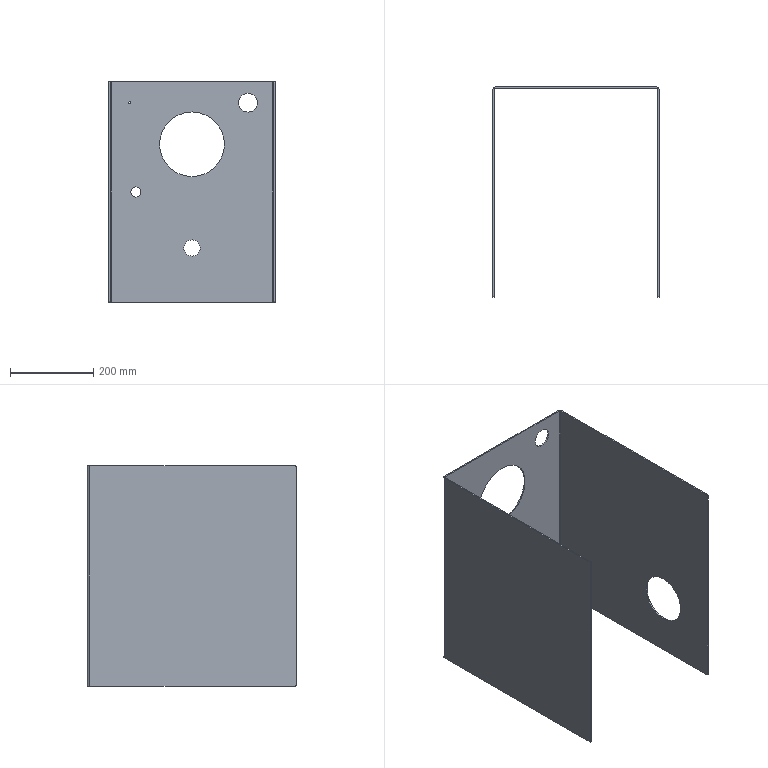Part | SolidWorks | features ICE 4, Cut 2, FlatPattern 1, SMBaseFlange 1, SheetMetal 1 | 1 solid | 38 faces | box 400 x 505 x 530 mm | volume 2126539 mm3 | cylinder 20 | plane 18 | commonest cylinder face diameters 6 x6 5.2 x2 12 x2 24.2 x2 39 x2 45.2 x2
STEP:
#1=CARTESIAN_POINT('',(397.,150.,208.7));
#2=VERTEX_POINT('',#1);
#3=CARTESIAN_POINT('',(397.,150.,91.3));
#4=VERTEX_POINT('',#3);
#5=CARTESIAN_POINT('',(397.,150.,150.));
#6=DIRECTION('',(1.,0.,0.));
#7=DIRECTION('',(0.,0.,-1.));
#8=AXIS2_PLACEMENT_3D('',#5,#6,#7);
#9=CIRCLE('',#8,58.7);
#10=EDGE_CURVE('',#2,#4,#9,.T.);
#11=ORIENTED_EDGE('',*,*,#10,.F.);
#12=CARTESIAN_POINT('',(400.,150.,208.7));
#13=VERTEX_POINT('',#12);
#14=CARTESIAN_POINT('',(390.,150.,208.7));
#15=DIRECTION('',(1.,0.,0.));
#16=VECTOR('',#15,1000.);
#17=LINE('',#14,#16);
#18=EDGE_CURVE('',#2,#13,#17,.T.);
#19=ORIENTED_EDGE('',*,*,#18,.T.);
#20=CARTESIAN_POINT('',(400.,150.,91.3));
#21=VERTEX_POINT('',#20);
#22=CARTESIAN_POINT('',(400.,150.,150.));
#23=DIRECTION('',(1.,0.,0.));
#24=DIRECTION('',(0.,0.,-1.));
#25=AXIS2_PLACEMENT_3D('',#22,#23,#24);
#26=CIRCLE('',#25,58.7);
#27=EDGE_CURVE('',#13,#21,#26,.T.);
#28=ORIENTED_EDGE('',*,*,#27,.T.);
#29=CARTESIAN_POINT('',(390.,150.,91.3));
#30=DIRECTION('',(1.,0.,0.));
#31=VECTOR('',#30,1000.);
#32=LINE('',#29,#31);
#33=EDGE_CURVE('',#4,#21,#32,.T.);
#34=ORIENTED_EDGE('',*,*,#33,.F.);
#35=EDGE_LOOP('',(#11,#19,#28,#34));
#36=FACE_OUTER_BOUND('',#35,.T.);
#37=CARTESIAN_POINT('',(390.,150.,150.));
#38=DIRECTION('',(1.,0.,0.));
#39=DIRECTION('',(0.,0.,-1.));
#40=AXIS2_PLACEMENT_3D('',#37,#38,#39);
#41=CYLINDRICAL_SURFACE('',#40,58.7);
#42=ADVANCED_FACE('',(#36),#41,.F.);
#43=CARTESIAN_POINT('',(200.,502.,302.));
#44=VERTEX_POINT('',#43);
#45=CARTESIAN_POINT('',(200.,502.,458.));
#46=VERTEX_POINT('',#45);
#47=CARTESIAN_POINT('',(200.,502.,380.));
#48=DIRECTION('',(0.,1.,0.));
#49=DIRECTION('',(0.,0.,1.));
#50=AXIS2_PLACEMENT_3D('',#47,#48,#49);
#51=CIRCLE('',#50,78.);
#52=EDGE_CURVE('',#44,#46,#51,.T.);
#53=ORIENTED_EDGE('',*,*,#52,.F.);
#54=CARTESIAN_POINT('',(200.,505.,302.));
#55=VERTEX_POINT('',#54);
#56=CARTESIAN_POINT('',(200.,495.,302.));
#57=DIRECTION('',(0.,1.,0.));
#58=VECTOR('',#57,1000.);
#59=LINE('',#56,#58);
#60=EDGE_CURVE('',#44,#55,#59,.T.);
#61=ORIENTED_EDGE('',*,*,#60,.T.);
#62=CARTESIAN_POINT('',(200.,505.,458.));
#63=VERTEX_POINT('',#62);
#64=CARTESIAN_POINT('',(200.,505.,380.));
#65=DIRECTION('',(0.,1.,0.));
#66=DIRECTION('',(0.,0.,1.));
#67=AXIS2_PLACEMENT_3D('',#64,#65,#66);
#68=CIRCLE('',#67,78.);
#69=EDGE_CURVE('',#55,#63,#68,.T.);
#70=ORIENTED_EDGE('',*,*,#69,.T.);
#71=CARTESIAN_POINT('',(200.,495.,458.));
#72=DIRECTION('',(0.,1.,0.));
#73=VECTOR('',#72,1000.);
#74=LINE('',#71,#73);
#75=EDGE_CURVE('',#46,#63,#74,.T.);
#76=ORIENTED_EDGE('',*,*,#75,.F.);
#77=EDGE_LOOP('',(#53,#61,#70,#76));
#78=FACE_OUTER_BOUND('',#77,.T.);
#79=CARTESIAN_POINT('',(200.,495.,380.));
#80=DIRECTION('',(0.,1.,0.));
#81=DIRECTION('',(0.,0.,1.));
#82=AXIS2_PLACEMENT_3D('',#79,#80,#81);
#83=CYLINDRICAL_SURFACE('',#82,78.);
#84=ADVANCED_FACE('',(#78),#83,.F.);
#85=CARTESIAN_POINT('',(50.,502.,477.4));
#86=VERTEX_POINT('',#85);
#87=CARTESIAN_POINT('',(50.,502.,482.6));
#88=VERTEX_POINT('',#87);
#89=CARTESIAN_POINT('',(50.,502.,480.));
#90=DIRECTION('',(0.,1.,0.));
#91=DIRECTION('',(0.,0.,1.));
#92=AXIS2_PLACEMENT_3D('',#89,#90,#91);
#93=CIRCLE('',#92,2.6);
#94=EDGE_CURVE('',#86,#88,#93,.T.);
#95=ORIENTED_EDGE('',*,*,#94,.F.);
#96=CARTESIAN_POINT('',(50.,505.,477.4));
#97=VERTEX_POINT('',#96);
#98=CARTESIAN_POINT('',(50.,495.,477.4));
#99=DIRECTION('',(0.,1.,0.));
#100=VECTOR('',#99,1000.);
#101=LINE('',#98,#100);
#102=EDGE_CURVE('',#86,#97,#101,.T.);
#103=ORIENTED_EDGE('',*,*,#102,.T.);
#104=CARTESIAN_POINT('',(50.,505.,482.6));
#105=VERTEX_POINT('',#104);
#106=CARTESIAN_POINT('',(50.,505.,480.));
#107=DIRECTION('',(0.,1.,0.));
#108=DIRECTION('',(0.,0.,1.));
#109=AXIS2_PLACEMENT_3D('',#106,#107,#108);
#110=CIRCLE('',#109,2.6);
#111=EDGE_CURVE('',#97,#105,#110,.T.);
#112=ORIENTED_EDGE('',*,*,#111,.T.);
#113=CARTESIAN_POINT('',(50.,495.,482.6));
#114=DIRECTION('',(0.,1.,0.));
#115=VECTOR('',#114,1000.);
#116=LINE('',#113,#115);
#117=EDGE_CURVE('',#88,#105,#116,.T.);
#118=ORIENTED_EDGE('',*,*,#117,.F.);
#119=EDGE_LOOP('',(#95,#103,#112,#118));
#120=FACE_OUTER_BOUND('',#119,.T.);
#121=CARTESIAN_POINT('',(50.,495.,480.));
#122=DIRECTION('',(0.,1.,0.));
#123=DIRECTION('',(0.,0.,1.));
#124=AXIS2_PLACEMENT_3D('',#121,#122,#123);
#125=CYLINDRICAL_SURFACE('',#124,2.6);
#126=ADVANCED_FACE('',(#120),#125,.F.);
#127=CARTESIAN_POINT('',(335.,502.,457.4));
#128=VERTEX_POINT('',#127);
#129=CARTESIAN_POINT('',(335.,502.,502.6));
#130=VERTEX_POINT('',#129);
#131=CARTESIAN_POINT('',(335.,502.,480.));
#132=DIRECTION('',(0.,1.,0.));
#133=DIRECTION('',(0.,0.,1.));
#134=AXIS2_PLACEMENT_3D('',#131,#132,#133);
#135=CIRCLE('',#134,22.6);
#136=EDGE_CURVE('',#128,#130,#135,.T.);
#137=ORIENTED_EDGE('',*,*,#136,.F.);
#138=CARTESIAN_POINT('',(335.,505.,457.4));
#139=VERTEX_POINT('',#138);
#140=CARTESIAN_POINT('',(335.,0.,457.4));
#141=DIRECTION('',(0.,1.,0.));
#142=VECTOR('',#141,1000.);
#143=LINE('',#140,#142);
#144=EDGE_CURVE('',#128,#139,#143,.T.);
#145=ORIENTED_EDGE('',*,*,#144,.T.);
#146=CARTESIAN_POINT('',(335.,505.,502.6));
#147=VERTEX_POINT('',#146);
#148=CARTESIAN_POINT('',(335.,505.,480.));
#149=DIRECTION('',(0.,1.,0.));
#150=DIRECTION('',(0.,0.,1.));
#151=AXIS2_PLACEMENT_3D('',#148,#149,#150);
#152=CIRCLE('',#151,22.6);
#153=EDGE_CURVE('',#139,#147,#152,.T.);
#154=ORIENTED_EDGE('',*,*,#153,.T.);
#155=CARTESIAN_POINT('',(335.,0.,502.6));
#156=DIRECTION('',(0.,1.,0.));
#157=VECTOR('',#156,1000.);
#158=LINE('',#155,#157);
#159=EDGE_CURVE('',#130,#147,#158,.T.);
#160=ORIENTED_EDGE('',*,*,#159,.F.);
#161=EDGE_LOOP('',(#137,#145,#154,#160));
#162=FACE_OUTER_BOUND('',#161,.T.);
#163=CARTESIAN_POINT('',(335.,0.,480.));
#164=DIRECTION('',(0.,1.,0.));
#165=DIRECTION('',(0.,0.,1.));
#166=AXIS2_PLACEMENT_3D('',#163,#164,#165);
#167=CYLINDRICAL_SURFACE('',#166,22.6);
#168=ADVANCED_FACE('',(#162),#167,.F.);
#169=CARTESIAN_POINT('',(65.,502.,252.9));
#170=VERTEX_POINT('',#169);
#171=CARTESIAN_POINT('',(65.,502.,277.1));
#172=VERTEX_POINT('',#171);
#173=CARTESIAN_POINT('',(65.,502.,265.));
#174=DIRECTION('',(0.,1.,0.));
#175=DIRECTION('',(0.,0.,1.));
#176=AXIS2_PLACEMENT_3D('',#173,#174,#175);
#177=CIRCLE('',#176,12.1);
#178=EDGE_CURVE('',#170,#172,#177,.T.);
#179=ORIENTED_EDGE('',*,*,#178,.F.);
#180=CARTESIAN_POINT('',(65.,505.,252.9));
#181=VERTEX_POINT('',#180);
#182=CARTESIAN_POINT('',(65.,0.,252.9));
#183=DIRECTION('',(0.,1.,0.));
#184=VECTOR('',#183,1000.);
#185=LINE('',#182,#184);
#186=EDGE_CURVE('',#170,#181,#185,.T.);
#187=ORIENTED_EDGE('',*,*,#186,.T.);
#188=CARTESIAN_POINT('',(65.,505.,277.1));
#189=VERTEX_POINT('',#188);
#190=CARTESIAN_POINT('',(65.,505.,265.));
#191=DIRECTION('',(0.,1.,0.));
#192=DIRECTION('',(0.,0.,1.));
#193=AXIS2_PLACEMENT_3D('',#190,#191,#192);
#194=CIRCLE('',#193,12.1);
#195=EDGE_CURVE('',#181,#189,#194,.T.);
#196=ORIENTED_EDGE('',*,*,#195,.T.);
#197=CARTESIAN_POINT('',(65.,0.,277.1));
#198=DIRECTION('',(0.,1.,0.));
#199=VECTOR('',#198,1000.);
#200=LINE('',#197,#199);
#201=EDGE_CURVE('',#172,#189,#200,.T.);
#202=ORIENTED_EDGE('',*,*,#201,.F.);
#203=EDGE_LOOP('',(#179,#187,#196,#202));
#204=FACE_OUTER_BOUND('',#203,.T.);
#205=CARTESIAN_POINT('',(65.,0.,265.));
#206=DIRECTION('',(0.,1.,0.));
#207=DIRECTION('',(0.,0.,1.));
#208=AXIS2_PLACEMENT_3D('',#205,#206,#207);
#209=CYLINDRICAL_SURFACE('',#208,12.1);
#210=ADVANCED_FACE('',(#204),#209,.F.);
#211=CARTESIAN_POINT('',(200.,502.,110.5));
#212=VERTEX_POINT('',#211);
#213=CARTESIAN_POINT('',(200.,502.,149.5));
#214=VERTEX_POINT('',#213);
#215=CARTESIAN_POINT('',(200.,502.,130.));
#216=DIRECTION('',(0.,1.,0.));
#217=DIRECTION('',(0.,0.,1.));
#218=AXIS2_PLACEMENT_3D('',#215,#216,#217);
#219=CIRCLE('',#218,19.5);
#220=EDGE_CURVE('',#212,#214,#219,.T.);
#221=ORIENTED_EDGE('',*,*,#220,.F.);
#222=CARTESIAN_POINT('',(200.,505.,110.5));
#223=VERTEX_POINT('',#222);
#224=CARTESIAN_POINT('',(200.,0.,110.5));
#225=DIRECTION('',(0.,1.,0.));
#226=VECTOR('',#225,1000.);
#227=LINE('',#224,#226);
#228=EDGE_CURVE('',#212,#223,#227,.T.);
#229=ORIENTED_EDGE('',*,*,#228,.T.);
#230=CARTESIAN_POINT('',(200.,505.,149.5));
#231=VERTEX_POINT('',#230);
#232=CARTESIAN_POINT('',(200.,505.,130.));
#233=DIRECTION('',(0.,1.,0.));
#234=DIRECTION('',(0.,0.,1.));
#235=AXIS2_PLACEMENT_3D('',#232,#233,#234);
#236=CIRCLE('',#235,19.5);
#237=EDGE_CURVE('',#223,#231,#236,.T.);
#238=ORIENTED_EDGE('',*,*,#237,.T.);
#239=CARTESIAN_POINT('',(200.,0.,149.5));
#240=DIRECTION('',(0.,1.,0.));
#241=VECTOR('',#240,1000.);
#242=LINE('',#239,#241);
#243=EDGE_CURVE('',#214,#231,#242,.T.);
#244=ORIENTED_EDGE('',*,*,#243,.F.);
#245=EDGE_LOOP('',(#221,#229,#238,#244));
#246=FACE_OUTER_BOUND('',#245,.T.);
#247=CARTESIAN_POINT('',(200.,0.,130.));
#248=DIRECTION('',(0.,1.,0.));
#249=DIRECTION('',(0.,0.,1.));
#250=AXIS2_PLACEMENT_3D('',#247,#248,#249);
#251=CYLINDRICAL_SURFACE('',#250,19.5);
#252=ADVANCED_FACE('',(#246),#251,.F.);
#253=CARTESIAN_POINT('',(397.,150.,150.));
#254=DIRECTION('',(1.,0.,0.));
#255=DIRECTION('',(0.,0.,-1.));
#256=AXIS2_PLACEMENT_3D('',#253,#254,#255);
#257=CIRCLE('',#256,58.7);
#258=EDGE_CURVE('',#4,#2,#257,.T.);
#259=ORIENTED_EDGE('',*,*,#258,.T.);
#260=ORIENTED_EDGE('',*,*,#10,.T.);
#261=EDGE_LOOP('',(#259,#260));
#262=FACE_BOUND('',#261,.T.);
#263=CARTESIAN_POINT('',(397.,0.,527.));
#264=VERTEX_POINT('',#263);
#265=CARTESIAN_POINT('',(397.,3.,530.));
#266=VERTEX_POINT('',#265);
#267=CARTESIAN_POINT('',(397.,3.,527.));
#268=DIRECTION('',(-1.,0.,0.));
#269=DIRECTION('',(0.,0.,-1.));
#270=AXIS2_PLACEMENT_3D('',#267,#268,#269);
#271=CIRCLE('',#270,3.);
#272=EDGE_CURVE('',#264,#266,#271,.T.);
#273=ORIENTED_EDGE('',*,*,#272,.T.);
#274=CARTESIAN_POINT('',(397.,499.,530.));
#275=VERTEX_POINT('',#274);
#276=CARTESIAN_POINT('',(397.,505.,530.));
#277=DIRECTION('',(0.,-1.,0.));
#278=VECTOR('',#277,1000.);
#279=LINE('',#276,#278);
#280=EDGE_CURVE('',#275,#266,#279,.T.);
#281=ORIENTED_EDGE('',*,*,#280,.F.);
#282=CARTESIAN_POINT('',(397.,499.,0.));
#283=VERTEX_POINT('',#282);
#284=CARTESIAN_POINT('',(397.,499.,530.));
#285=DIRECTION('',(0.,0.,-1.));
#286=VECTOR('',#285,1000.);
#287=LINE('',#284,#286);
#288=EDGE_CURVE('',#275,#283,#287,.T.);
#289=ORIENTED_EDGE('',*,*,#288,.T.);
#290=CARTESIAN_POINT('',(397.,3.,0.));
#291=VERTEX_POINT('',#290);
#292=CARTESIAN_POINT('',(397.,505.,0.));
#293=DIRECTION('',(0.,-1.,0.));
#294=VECTOR('',#293,1000.);
#295=LINE('',#292,#294);
#296=EDGE_CURVE('',#283,#291,#295,.T.);
#297=ORIENTED_EDGE('',*,*,#296,.T.);
#298=CARTESIAN_POINT('',(397.,0.,3.));
#299=VERTEX_POINT('',#298);
#300=CARTESIAN_POINT('',(397.,3.,3.));
#301=DIRECTION('',(-1.,0.,0.));
#302=DIRECTION('',(0.,0.,-1.));
#303=AXIS2_PLACEMENT_3D('',#300,#301,#302);
#304=CIRCLE('',#303,3.);
#305=EDGE_CURVE('',#291,#299,#304,.T.);
#306=ORIENTED_EDGE('',*,*,#305,.T.);
#307=CARTESIAN_POINT('',(397.,0.,530.));
#308=DIRECTION('',(0.,0.,-1.));
#309=VECTOR('',#308,1000.);
#310=LINE('',#307,#309);
#311=EDGE_CURVE('',#264,#299,#310,.T.);
#312=ORIENTED_EDGE('',*,*,#311,.F.);
#313=EDGE_LOOP('',(#273,#281,#289,#297,#306,#312));
#314=FACE_OUTER_BOUND('',#313,.T.);
#315=CARTESIAN_POINT('',(397.,505.,530.));
#316=DIRECTION('',(1.,0.,0.));
#317=DIRECTION('',(0.,0.,-1.));
#318=AXIS2_PLACEMENT_3D('',#315,#316,#317);
#319=PLANE('',#318);
#320=ADVANCED_FACE('',(#262,#314),#319,.F.);
#321=CARTESIAN_POINT('',(400.,150.,150.));
#322=DIRECTION('',(1.,0.,0.));
#323=DIRECTION('',(0.,0.,-1.));
#324=AXIS2_PLACEMENT_3D('',#321,#322,#323);
#325=CIRCLE('',#324,58.7);
#326=EDGE_CURVE('',#21,#13,#325,.T.);
#327=ORIENTED_EDGE('',*,*,#326,.F.);
#328=ORIENTED_EDGE('',*,*,#27,.F.);
#329=EDGE_LOOP('',(#327,#328));
#330=FACE_BOUND('',#329,.T.);
#331=CARTESIAN_POINT('',(400.,499.,530.));
#332=VERTEX_POINT('',#331);
#333=CARTESIAN_POINT('',(400.,3.,530.));
#334=VERTEX_POINT('',#333);
#335=CARTESIAN_POINT('',(400.,505.,530.));
#336=DIRECTION('',(0.,-1.,0.));
#337=VECTOR('',#336,1000.);
#338=LINE('',#335,#337);
#339=EDGE_CURVE('',#332,#334,#338,.T.);
#340=ORIENTED_EDGE('',*,*,#339,.T.);
#341=CARTESIAN_POINT('',(400.,0.,527.));
#342=VERTEX_POINT('',#341);
#343=CARTESIAN_POINT('',(400.,3.,527.));
#344=DIRECTION('',(-1.,0.,0.));
#345=DIRECTION('',(0.,0.,-1.));
#346=AXIS2_PLACEMENT_3D('',#343,#344,#345);
#347=CIRCLE('',#346,3.);
#348=EDGE_CURVE('',#342,#334,#347,.T.);
#349=ORIENTED_EDGE('',*,*,#348,.F.);
#350=CARTESIAN_POINT('',(400.,0.,3.));
#351=VERTEX_POINT('',#350);
#352=CARTESIAN_POINT('',(400.,0.,530.));
#353=DIRECTION('',(0.,0.,-1.));
#354=VECTOR('',#353,1000.);
#355=LINE('',#352,#354);
#356=EDGE_CURVE('',#342,#351,#355,.T.);
#357=ORIENTED_EDGE('',*,*,#356,.T.);
#358=CARTESIAN_POINT('',(400.,3.,0.));
#359=VERTEX_POINT('',#358);
#360=CARTESIAN_POINT('',(400.,3.,3.));
#361=DIRECTION('',(-1.,0.,0.));
#362=DIRECTION('',(0.,0.,-1.));
#363=AXIS2_PLACEMENT_3D('',#360,#361,#362);
#364=CIRCLE('',#363,3.);
#365=EDGE_CURVE('',#359,#351,#364,.T.);
#366=ORIENTED_EDGE('',*,*,#365,.F.);
#367=CARTESIAN_POINT('',(400.,499.,0.));
#368=VERTEX_POINT('',#367);
#369=CARTESIAN_POINT('',(400.,505.,0.));
#370=DIRECTION('',(0.,-1.,0.));
#371=VECTOR('',#370,1000.);
#372=LINE('',#369,#371);
#373=EDGE_CURVE('',#368,#359,#372,.T.);
#374=ORIENTED_EDGE('',*,*,#373,.F.);
#375=CARTESIAN_POINT('',(400.,499.,530.));
#376=DIRECTION('',(0.,0.,-1.));
#377=VECTOR('',#376,1000.);
#378=LINE('',#375,#377);
#379=EDGE_CURVE('',#332,#368,#378,.T.);
#380=ORIENTED_EDGE('',*,*,#379,.F.);
#381=EDGE_LOOP('',(#340,#349,#357,#366,#374,#380));
#382=FACE_OUTER_BOUND('',#381,.T.);
#383=CARTESIAN_POINT('',(400.,505.,530.));
#384=DIRECTION('',(1.,0.,0.));
#385=DIRECTION('',(0.,0.,-1.));
#386=AXIS2_PLACEMENT_3D('',#383,#384,#385);
#387=PLANE('',#386);
#388=ADVANCED_FACE('',(#330,#382),#387,.T.);
#389=ORIENTED_EDGE('',*,*,#280,.T.);
#390=CARTESIAN_POINT('',(397.,3.,530.));
#391=DIRECTION('',(1.,0.,0.));
#392=VECTOR('',#391,1000.);
#393=LINE('',#390,#392);
#394=EDGE_CURVE('',#266,#334,#393,.T.);
#395=ORIENTED_EDGE('',*,*,#394,.T.);
#396=ORIENTED_EDGE('',*,*,#339,.F.);
#397=CARTESIAN_POINT('',(400.,499.,530.));
#398=DIRECTION('',(-1.,0.,0.));
#399=VECTOR('',#398,1000.);
#400=LINE('',#397,#399);
#401=EDGE_CURVE('',#332,#275,#400,.T.);
#402=ORIENTED_EDGE('',*,*,#401,.T.);
#403=EDGE_LOOP('',(#389,#395,#396,#402));
#404=FACE_OUTER_BOUND('',#403,.T.);
#405=CARTESIAN_POINT('',(394.,502.,530.));
#406=DIRECTION('',(0.,0.,1.));
#407=DIRECTION('',(1.,0.,0.));
#408=AXIS2_PLACEMENT_3D('',#405,#406,#407);
#409=PLANE('',#408);
#410=ADVANCED_FACE('',(#404),#409,.T.);
#411=CARTESIAN_POINT('',(397.,0.,527.));
#412=DIRECTION('',(1.,0.,0.));
#413=VECTOR('',#412,1000.);
#414=LINE('',#411,#413);
#415=EDGE_CURVE('',#264,#342,#414,.T.);
#416=ORIENTED_EDGE('',*,*,#415,.F.);
#417=ORIENTED_EDGE('',*,*,#311,.T.);
#418=CARTESIAN_POINT('',(397.,0.,3.));
#419=DIRECTION('',(1.,0.,0.));
#420=VECTOR('',#419,1000.);
#421=LINE('',#418,#420);
#422=EDGE_CURVE('',#299,#351,#421,.T.);
#423=ORIENTED_EDGE('',*,*,#422,.T.);
#424=ORIENTED_EDGE('',*,*,#356,.F.);
#425=EDGE_LOOP('',(#416,#417,#423,#424));
#426=FACE_OUTER_BOUND('',#425,.T.);
#427=CARTESIAN_POINT('',(400.,0.,530.));
#428=DIRECTION('',(0.,-1.,0.));
#429=DIRECTION('',(0.,0.,-1.));
#430=AXIS2_PLACEMENT_3D('',#427,#428,#429);
#431=PLANE('',#430);
#432=ADVANCED_FACE('',(#426),#431,.T.);
#433=CARTESIAN_POINT('',(397.,3.,0.));
#434=DIRECTION('',(1.,0.,0.));
#435=VECTOR('',#434,1000.);
#436=LINE('',#433,#435);
#437=EDGE_CURVE('',#291,#359,#436,.T.);
#438=ORIENTED_EDGE('',*,*,#437,.F.);
#439=ORIENTED_EDGE('',*,*,#296,.F.);
#440=CARTESIAN_POINT('',(397.,499.,0.));
#441=DIRECTION('',(1.,0.,0.));
#442=VECTOR('',#441,1000.);
#443=LINE('',#440,#442);
#444=EDGE_CURVE('',#283,#368,#443,.T.);
#445=ORIENTED_EDGE('',*,*,#444,.T.);
#446=ORIENTED_EDGE('',*,*,#373,.T.);
#447=EDGE_LOOP('',(#438,#439,#445,#446));
#448=FACE_OUTER_BOUND('',#447,.T.);
#449=CARTESIAN_POINT('',(394.,499.,0.));
#450=DIRECTION('',(0.,0.,1.));
#451=DIRECTION('',(1.,0.,0.));
#452=AXIS2_PLACEMENT_3D('',#449,#450,#451);
#453=PLANE('',#452);
#454=ADVANCED_FACE('',(#448),#453,.F.);
#455=CARTESIAN_POINT('',(0.,0.,527.));
#456=VERTEX_POINT('',#455);
#457=CARTESIAN_POINT('',(0.,0.,3.));
#458=VERTEX_POINT('',#457);
#459=CARTESIAN_POINT('',(0.,0.,530.));
#460=DIRECTION('',(0.,0.,-1.));
#461=VECTOR('',#460,1000.);
#462=LINE('',#459,#461);
#463=EDGE_CURVE('',#456,#458,#462,.T.);
#464=ORIENTED_EDGE('',*,*,#463,.F.);
#465=CARTESIAN_POINT('',(0.,3.,530.));
#466=VERTEX_POINT('',#465);
#467=CARTESIAN_POINT('',(0.,3.,527.));
#468=DIRECTION('',(1.,0.,0.));
#469=DIRECTION('',(0.,0.,1.));
#470=AXIS2_PLACEMENT_3D('',#467,#468,#469);
#471=CIRCLE('',#470,3.);
#472=EDGE_CURVE('',#466,#456,#471,.T.);
#473=ORIENTED_EDGE('',*,*,#472,.F.);
#474=CARTESIAN_POINT('',(0.,499.,530.));
#475=VERTEX_POINT('',#474);
#476=CARTESIAN_POINT('',(0.,0.,530.));
#477=DIRECTION('',(0.,1.,0.));
#478=VECTOR('',#477,1000.);
#479=LINE('',#476,#478);
#480=EDGE_CURVE('',#466,#475,#479,.T.);
#481=ORIENTED_EDGE('',*,*,#480,.T.);
#482=CARTESIAN_POINT('',(0.,499.,0.));
#483=VERTEX_POINT('',#482);
#484=CARTESIAN_POINT('',(0.,499.,530.));
#485=DIRECTION('',(0.,0.,-1.));
#486=VECTOR('',#485,1000.);
#487=LINE('',#484,#486);
#488=EDGE_CURVE('',#475,#483,#487,.T.);
#489=ORIENTED_EDGE('',*,*,#488,.T.);
#490=CARTESIAN_POINT('',(0.,3.,0.));
#491=VERTEX_POINT('',#490);
#492=CARTESIAN_POINT('',(0.,0.,0.));
#493=DIRECTION('',(0.,1.,0.));
#494=VECTOR('',#493,1000.);
#495=LINE('',#492,#494);
#496=EDGE_CURVE('',#491,#483,#495,.T.);
#497=ORIENTED_EDGE('',*,*,#496,.F.);
#498=CARTESIAN_POINT('',(0.,3.,3.));
#499=DIRECTION('',(1.,0.,0.));
#500=DIRECTION('',(0.,0.,1.));
#501=AXIS2_PLACEMENT_3D('',#498,#499,#500);
#502=CIRCLE('',#501,3.);
#503=EDGE_CURVE('',#458,#491,#502,.T.);
#504=ORIENTED_EDGE('',*,*,#503,.F.);
#505=EDGE_LOOP('',(#464,#473,#481,#489,#497,#504));
#506=FACE_OUTER_BOUND('',#505,.T.);
#507=CARTESIAN_POINT('',(0.,0.,530.));
#508=DIRECTION('',(-1.,0.,0.));
#509=DIRECTION('',(0.,0.,1.));
#510=AXIS2_PLACEMENT_3D('',#507,#508,#509);
#511=PLANE('',#510);
#512=ADVANCED_FACE('',(#506),#511,.T.);
#513=CARTESIAN_POINT('',(3.,3.,530.));
#514=VERTEX_POINT('',#513);
#515=CARTESIAN_POINT('',(3.,0.,527.));
#516=VERTEX_POINT('',#515);
#517=CARTESIAN_POINT('',(3.,3.,527.));
#518=DIRECTION('',(1.,0.,0.));
#519=DIRECTION('',(0.,0.,1.));
#520=AXIS2_PLACEMENT_3D('',#517,#518,#519);
#521=CIRCLE('',#520,3.);
#522=EDGE_CURVE('',#514,#516,#521,.T.);
#523=ORIENTED_EDGE('',*,*,#522,.T.);
#524=CARTESIAN_POINT('',(3.,0.,3.));
#525=VERTEX_POINT('',#524);
#526=CARTESIAN_POINT('',(3.,0.,530.));
#527=DIRECTION('',(0.,0.,-1.));
#528=VECTOR('',#527,1000.);
#529=LINE('',#526,#528);
#530=EDGE_CURVE('',#516,#525,#529,.T.);
#531=ORIENTED_EDGE('',*,*,#530,.T.);
#532=CARTESIAN_POINT('',(3.,3.,0.));
#533=VERTEX_POINT('',#532);
#534=CARTESIAN_POINT('',(3.,3.,3.));
#535=DIRECTION('',(1.,0.,0.));
#536=DIRECTION('',(0.,0.,1.));
#537=AXIS2_PLACEMENT_3D('',#534,#535,#536);
#538=CIRCLE('',#537,3.);
#539=EDGE_CURVE('',#525,#533,#538,.T.);
#540=ORIENTED_EDGE('',*,*,#539,.T.);
#541=CARTESIAN_POINT('',(3.,499.,0.));
#542=VERTEX_POINT('',#541);
#543=CARTESIAN_POINT('',(3.,0.,0.));
#544=DIRECTION('',(0.,1.,0.));
#545=VECTOR('',#544,1000.);
#546=LINE('',#543,#545);
#547=EDGE_CURVE('',#533,#542,#546,.T.);
#548=ORIENTED_EDGE('',*,*,#547,.T.);
#549=CARTESIAN_POINT('',(3.,499.,530.));
#550=VERTEX_POINT('',#549);
#551=CARTESIAN_POINT('',(3.,499.,530.));
#552=DIRECTION('',(0.,0.,-1.));
#553=VECTOR('',#552,1000.);
#554=LINE('',#551,#553);
#555=EDGE_CURVE('',#550,#542,#554,.T.);
#556=ORIENTED_EDGE('',*,*,#555,.F.);
#557=CARTESIAN_POINT('',(3.,0.,530.));
#558=DIRECTION('',(0.,1.,0.));
#559=VECTOR('',#558,1000.);
#560=LINE('',#557,#559);
#561=EDGE_CURVE('',#514,#550,#560,.T.);
#562=ORIENTED_EDGE('',*,*,#561,.F.);
#563=EDGE_LOOP('',(#523,#531,#540,#548,#556,#562));
#564=FACE_OUTER_BOUND('',#563,.T.);
#565=CARTESIAN_POINT('',(3.,0.,530.));
#566=DIRECTION('',(-1.,0.,0.));
#567=DIRECTION('',(0.,0.,1.));
#568=AXIS2_PLACEMENT_3D('',#565,#566,#567);
#569=PLANE('',#568);
#570=ADVANCED_FACE('',(#564),#569,.F.);
#571=ORIENTED_EDGE('',*,*,#530,.F.);
#572=CARTESIAN_POINT('',(3.,0.,527.));
#573=DIRECTION('',(-1.,0.,0.));
#574=VECTOR('',#573,1000.);
#575=LINE('',#572,#574);
#576=EDGE_CURVE('',#516,#456,#575,.T.);
#577=ORIENTED_EDGE('',*,*,#576,.T.);
#578=ORIENTED_EDGE('',*,*,#463,.T.);
#579=CARTESIAN_POINT('',(3.,0.,3.));
#580=DIRECTION('',(-1.,0.,0.));
#581=VECTOR('',#580,1000.);
#582=LINE('',#579,#581);
#583=EDGE_CURVE('',#525,#458,#582,.T.);
#584=ORIENTED_EDGE('',*,*,#583,.F.);
#585=EDGE_LOOP('',(#571,#577,#578,#584));
#586=FACE_OUTER_BOUND('',#585,.T.);
#587=CARTESIAN_POINT('',(3.,0.,530.));
#588=DIRECTION('',(0.,-1.,0.));
#589=DIRECTION('',(0.,0.,-1.));
#590=AXIS2_PLACEMENT_3D('',#587,#588,#589);
#591=PLANE('',#590);
#592=ADVANCED_FACE('',(#586),#591,.T.);
#593=ORIENTED_EDGE('',*,*,#547,.F.);
#594=CARTESIAN_POINT('',(3.,3.,0.));
#595=DIRECTION('',(-1.,0.,0.));
#596=VECTOR('',#595,1000.);
#597=LINE('',#594,#596);
#598=EDGE_CURVE('',#533,#491,#597,.T.);
#599=ORIENTED_EDGE('',*,*,#598,.T.);
#600=ORIENTED_EDGE('',*,*,#496,.T.);
#601=CARTESIAN_POINT('',(0.,499.,0.));
#602=DIRECTION('',(1.,0.,0.));
#603=VECTOR('',#602,1000.);
#604=LINE('',#601,#603);
#605=EDGE_CURVE('',#483,#542,#604,.T.);
#606=ORIENTED_EDGE('',*,*,#605,.T.);
#607=EDGE_LOOP('',(#593,#599,#600,#606));
#608=FACE_OUTER_BOUND('',#607,.T.);
#609=CARTESIAN_POINT('',(6.,502.,0.));
#610=DIRECTION('',(0.,0.,-1.));
#611=DIRECTION('',(-1.,0.,0.));
#612=AXIS2_PLACEMENT_3D('',#609,#610,#611);
#613=PLANE('',#612);
#614=ADVANCED_FACE('',(#608),#613,.T.);
#615=CARTESIAN_POINT('',(6.,505.,530.));
#616=VERTEX_POINT('',#615);
#617=CARTESIAN_POINT('',(6.,502.,530.));
#618=VERTEX_POINT('',#617);
#619=CARTESIAN_POINT('',(6.,505.,530.));
#620=DIRECTION('',(0.,-1.,0.));
#621=VECTOR('',#620,1000.);
#622=LINE('',#619,#621);
#623=EDGE_CURVE('',#616,#618,#622,.T.);
#624=ORIENTED_EDGE('',*,*,#623,.F.);
#625=CARTESIAN_POINT('',(6.,499.,530.));
#626=DIRECTION('',(0.,0.,-1.));
#627=DIRECTION('',(1.,0.,0.));
#628=AXIS2_PLACEMENT_3D('',#625,#626,#627);
#629=CIRCLE('',#628,6.);
#630=EDGE_CURVE('',#475,#616,#629,.T.);
#631=ORIENTED_EDGE('',*,*,#630,.F.);
#632=CARTESIAN_POINT('',(3.,499.,530.));
#633=DIRECTION('',(-1.,0.,0.));
#634=VECTOR('',#633,1000.);
#635=LINE('',#632,#634);
#636=EDGE_CURVE('',#550,#475,#635,.T.);
#637=ORIENTED_EDGE('',*,*,#636,.F.);
#638=CARTESIAN_POINT('',(6.,499.,530.));
#639=DIRECTION('',(0.,0.,-1.));
#640=DIRECTION('',(1.,0.,0.));
#641=AXIS2_PLACEMENT_3D('',#638,#639,#640);
#642=CIRCLE('',#641,3.);
#643=EDGE_CURVE('',#550,#618,#642,.T.);
#644=ORIENTED_EDGE('',*,*,#643,.T.);
#645=EDGE_LOOP('',(#624,#631,#637,#644));
#646=FACE_OUTER_BOUND('',#645,.T.);
#647=CARTESIAN_POINT('',(6.,505.,530.));
#648=DIRECTION('',(0.,0.,1.));
#649=DIRECTION('',(1.,0.,0.));
#650=AXIS2_PLACEMENT_3D('',#647,#648,#649);
#651=PLANE('',#650);
#652=ADVANCED_FACE('',(#646),#651,.T.);
#653=CARTESIAN_POINT('',(394.,505.,530.));
#654=VERTEX_POINT('',#653);
#655=CARTESIAN_POINT('',(0.,505.,530.));
#656=DIRECTION('',(1.,0.,0.));
#657=VECTOR('',#656,1000.);
#658=LINE('',#655,#657);
#659=EDGE_CURVE('',#616,#654,#658,.T.);
#660=ORIENTED_EDGE('',*,*,#659,.F.);
#661=ORIENTED_EDGE('',*,*,#623,.T.);
#662=CARTESIAN_POINT('',(394.,502.,530.));
#663=VERTEX_POINT('',#662);
#664=CARTESIAN_POINT('',(0.,502.,530.));
#665=DIRECTION('',(1.,0.,0.));
#666=VECTOR('',#665,1000.);
#667=LINE('',#664,#666);
#668=EDGE_CURVE('',#618,#663,#667,.T.);
#669=ORIENTED_EDGE('',*,*,#668,.T.);
#670=CARTESIAN_POINT('',(394.,502.,530.));
#671=DIRECTION('',(0.,1.,0.));
#672=VECTOR('',#671,1000.);
#673=LINE('',#670,#672);
#674=EDGE_CURVE('',#663,#654,#673,.T.);
#675=ORIENTED_EDGE('',*,*,#674,.T.);
#676=EDGE_LOOP('',(#660,#661,#669,#675));
#677=FACE_OUTER_BOUND('',#676,.T.);
#678=CARTESIAN_POINT('',(3.,499.,530.));
#679=DIRECTION('',(0.,0.,1.));
#680=DIRECTION('',(1.,0.,0.));
#681=AXIS2_PLACEMENT_3D('',#678,#679,#680);
#682=PLANE('',#681);
#683=ADVANCED_FACE('',(#677),#682,.T.);
#684=ORIENTED_EDGE('',*,*,#605,.F.);
#685=CARTESIAN_POINT('',(6.,505.,0.));
#686=VERTEX_POINT('',#685);
#687=CARTESIAN_POINT('',(6.,499.,0.));
#688=DIRECTION('',(0.,0.,-1.));
#689=DIRECTION('',(1.,0.,0.));
#690=AXIS2_PLACEMENT_3D('',#687,#688,#689);
#691=CIRCLE('',#690,6.);
#692=EDGE_CURVE('',#483,#686,#691,.T.);
#693=ORIENTED_EDGE('',*,*,#692,.T.);
#694=CARTESIAN_POINT('',(6.,502.,0.));
#695=VERTEX_POINT('',#694);
#696=CARTESIAN_POINT('',(6.,502.,0.));
#697=DIRECTION('',(0.,1.,0.));
#698=VECTOR('',#697,1000.);
#699=LINE('',#696,#698);
#700=EDGE_CURVE('',#695,#686,#699,.T.);
#701=ORIENTED_EDGE('',*,*,#700,.F.);
#702=CARTESIAN_POINT('',(6.,499.,0.));
#703=DIRECTION('',(0.,0.,-1.));
#704=DIRECTION('',(1.,0.,0.));
#705=AXIS2_PLACEMENT_3D('',#702,#703,#704);
#706=CIRCLE('',#705,3.);
#707=EDGE_CURVE('',#542,#695,#706,.T.);
#708=ORIENTED_EDGE('',*,*,#707,.F.);
#709=EDGE_LOOP('',(#684,#693,#701,#708));
#710=FACE_OUTER_BOUND('',#709,.T.);
#711=CARTESIAN_POINT('',(0.,499.,0.));
#712=DIRECTION('',(0.,0.,-1.));
#713=DIRECTION('',(-1.,0.,0.));
#714=AXIS2_PLACEMENT_3D('',#711,#712,#713);
#715=PLANE('',#714);
#716=ADVANCED_FACE('',(#710),#715,.T.);
#717=ORIENTED_EDGE('',*,*,#401,.F.);
#718=CARTESIAN_POINT('',(394.,499.,530.));
#719=DIRECTION('',(0.,0.,-1.));
#720=DIRECTION('',(1.,0.,0.));
#721=AXIS2_PLACEMENT_3D('',#718,#719,#720);
#722=CIRCLE('',#721,6.);
#723=EDGE_CURVE('',#654,#332,#722,.T.);
#724=ORIENTED_EDGE('',*,*,#723,.F.);
#725=ORIENTED_EDGE('',*,*,#674,.F.);
#726=CARTESIAN_POINT('',(394.,499.,530.));
#727=DIRECTION('',(0.,0.,-1.));
#728=DIRECTION('',(1.,0.,0.));
#729=AXIS2_PLACEMENT_3D('',#726,#727,#728);
#730=CIRCLE('',#729,3.);
#731=EDGE_CURVE('',#663,#275,#730,.T.);
#732=ORIENTED_EDGE('',*,*,#731,.T.);
#733=EDGE_LOOP('',(#717,#724,#725,#732));
#734=FACE_OUTER_BOUND('',#733,.T.);
#735=CARTESIAN_POINT('',(400.,499.,530.));
#736=DIRECTION('',(0.,0.,1.));
#737=DIRECTION('',(1.,0.,0.));
#738=AXIS2_PLACEMENT_3D('',#735,#736,#737);
#739=PLANE('',#738);
#740=ADVANCED_FACE('',(#734),#739,.T.);
#741=CARTESIAN_POINT('',(394.,505.,0.));
#742=VERTEX_POINT('',#741);
#743=CARTESIAN_POINT('',(394.,502.,0.));
#744=VERTEX_POINT('',#743);
#745=CARTESIAN_POINT('',(394.,505.,0.));
#746=DIRECTION('',(0.,-1.,0.));
#747=VECTOR('',#746,1000.);
#748=LINE('',#745,#747);
#749=EDGE_CURVE('',#742,#744,#748,.T.);
#750=ORIENTED_EDGE('',*,*,#749,.F.);
#751=CARTESIAN_POINT('',(394.,499.,0.));
#752=DIRECTION('',(0.,0.,-1.));
#753=DIRECTION('',(1.,0.,0.));
#754=AXIS2_PLACEMENT_3D('',#751,#752,#753);
#755=CIRCLE('',#754,6.);
#756=EDGE_CURVE('',#742,#368,#755,.T.);
#757=ORIENTED_EDGE('',*,*,#756,.T.);
#758=ORIENTED_EDGE('',*,*,#444,.F.);
#759=CARTESIAN_POINT('',(394.,499.,0.));
#760=DIRECTION('',(0.,0.,-1.));
#761=DIRECTION('',(1.,0.,0.));
#762=AXIS2_PLACEMENT_3D('',#759,#760,#761);
#763=CIRCLE('',#762,3.);
#764=EDGE_CURVE('',#744,#283,#763,.T.);
#765=ORIENTED_EDGE('',*,*,#764,.F.);
#766=EDGE_LOOP('',(#750,#757,#758,#765));
#767=FACE_OUTER_BOUND('',#766,.T.);
#768=CARTESIAN_POINT('',(394.,505.,0.));
#769=DIRECTION('',(0.,0.,-1.));
#770=DIRECTION('',(-1.,0.,0.));
#771=AXIS2_PLACEMENT_3D('',#768,#769,#770);
#772=PLANE('',#771);
#773=ADVANCED_FACE('',(#767),#772,.T.);
#774=CARTESIAN_POINT('',(0.,505.,0.));
#775=DIRECTION('',(1.,0.,0.));
#776=VECTOR('',#775,1000.);
#777=LINE('',#774,#776);
#778=EDGE_CURVE('',#686,#742,#777,.T.);
#779=ORIENTED_EDGE('',*,*,#778,.T.);
#780=ORIENTED_EDGE('',*,*,#749,.T.);
#781=CARTESIAN_POINT('',(0.,502.,0.));
#782=DIRECTION('',(1.,0.,0.));
#783=VECTOR('',#782,1000.);
#784=LINE('',#781,#783);
#785=EDGE_CURVE('',#695,#744,#784,.T.);
#786=ORIENTED_EDGE('',*,*,#785,.F.);
#787=ORIENTED_EDGE('',*,*,#700,.T.);
#788=EDGE_LOOP('',(#779,#780,#786,#787));
#789=FACE_OUTER_BOUND('',#788,.T.);
#790=CARTESIAN_POINT('',(397.,499.,0.));
#791=DIRECTION('',(0.,0.,-1.));
#792=DIRECTION('',(-1.,0.,0.));
#793=AXIS2_PLACEMENT_3D('',#790,#791,#792);
#794=PLANE('',#793);
#795=ADVANCED_FACE('',(#789),#794,.T.);
#796=ORIENTED_EDGE('',*,*,#756,.F.);
#797=CARTESIAN_POINT('',(394.,505.,530.));
#798=DIRECTION('',(0.,0.,-1.));
#799=VECTOR('',#798,1000.);
#800=LINE('',#797,#799);
#801=EDGE_CURVE('',#654,#742,#800,.T.);
#802=ORIENTED_EDGE('',*,*,#801,.F.);
#803=ORIENTED_EDGE('',*,*,#723,.T.);
#804=ORIENTED_EDGE('',*,*,#379,.T.);
#805=EDGE_LOOP('',(#796,#802,#803,#804));
#806=FACE_OUTER_BOUND('',#805,.T.);
#807=CARTESIAN_POINT('',(394.,499.,530.));
#808=DIRECTION('',(0.,0.,-1.));
#809=DIRECTION('',(-1.,0.,0.));
#810=AXIS2_PLACEMENT_3D('',#807,#808,#809);
#811=CYLINDRICAL_SURFACE('',#810,6.);
#812=ADVANCED_FACE('',(#806),#811,.T.);
#813=CARTESIAN_POINT('',(200.,505.,380.));
#814=DIRECTION('',(0.,1.,0.));
#815=DIRECTION('',(0.,0.,1.));
#816=AXIS2_PLACEMENT_3D('',#813,#814,#815);
#817=CIRCLE('',#816,78.);
#818=EDGE_CURVE('',#63,#55,#817,.T.);
#819=ORIENTED_EDGE('',*,*,#818,.F.);
#820=ORIENTED_EDGE('',*,*,#69,.F.);
#821=EDGE_LOOP('',(#819,#820));
#822=FACE_BOUND('',#821,.T.);
#823=CARTESIAN_POINT('',(50.,505.,480.));
#824=DIRECTION('',(0.,1.,0.));
#825=DIRECTION('',(0.,0.,1.));
#826=AXIS2_PLACEMENT_3D('',#823,#824,#825);
#827=CIRCLE('',#826,2.6);
#828=EDGE_CURVE('',#105,#97,#827,.T.);
#829=ORIENTED_EDGE('',*,*,#828,.F.);
#830=ORIENTED_EDGE('',*,*,#111,.F.);
#831=EDGE_LOOP('',(#829,#830));
#832=FACE_BOUND('',#831,.T.);
#833=CARTESIAN_POINT('',(335.,505.,480.));
#834=DIRECTION('',(0.,1.,0.));
#835=DIRECTION('',(0.,0.,1.));
#836=AXIS2_PLACEMENT_3D('',#833,#834,#835);
#837=CIRCLE('',#836,22.6);
#838=EDGE_CURVE('',#147,#139,#837,.T.);
#839=ORIENTED_EDGE('',*,*,#838,.F.);
#840=ORIENTED_EDGE('',*,*,#153,.F.);
#841=EDGE_LOOP('',(#839,#840));
#842=FACE_BOUND('',#841,.T.);
#843=CARTESIAN_POINT('',(65.,505.,265.));
#844=DIRECTION('',(0.,1.,0.));
#845=DIRECTION('',(0.,0.,1.));
#846=AXIS2_PLACEMENT_3D('',#843,#844,#845);
#847=CIRCLE('',#846,12.1);
#848=EDGE_CURVE('',#189,#181,#847,.T.);
#849=ORIENTED_EDGE('',*,*,#848,.F.);
#850=ORIENTED_EDGE('',*,*,#195,.F.);
#851=EDGE_LOOP('',(#849,#850));
#852=FACE_BOUND('',#851,.T.);
#853=CARTESIAN_POINT('',(200.,505.,130.));
#854=DIRECTION('',(0.,1.,0.));
#855=DIRECTION('',(0.,0.,1.));
#856=AXIS2_PLACEMENT_3D('',#853,#854,#855);
#857=CIRCLE('',#856,19.5);
#858=EDGE_CURVE('',#231,#223,#857,.T.);
#859=ORIENTED_EDGE('',*,*,#858,.F.);
#860=ORIENTED_EDGE('',*,*,#237,.F.);
#861=EDGE_LOOP('',(#859,#860));
#862=FACE_BOUND('',#861,.T.);
#863=ORIENTED_EDGE('',*,*,#778,.F.);
#864=CARTESIAN_POINT('',(6.,505.,530.));
#865=DIRECTION('',(0.,0.,-1.));
#866=VECTOR('',#865,1000.);
#867=LINE('',#864,#866);
#868=EDGE_CURVE('',#616,#686,#867,.T.);
#869=ORIENTED_EDGE('',*,*,#868,.F.);
#870=ORIENTED_EDGE('',*,*,#659,.T.);
#871=ORIENTED_EDGE('',*,*,#801,.T.);
#872=EDGE_LOOP('',(#863,#869,#870,#871));
#873=FACE_OUTER_BOUND('',#872,.T.);
#874=CARTESIAN_POINT('',(0.,505.,530.));
#875=DIRECTION('',(0.,1.,0.));
#876=DIRECTION('',(0.,0.,1.));
#877=AXIS2_PLACEMENT_3D('',#874,#875,#876);
#878=PLANE('',#877);
#879=ADVANCED_FACE('',(#822,#832,#842,#852,#862,#873),#878,.T.);
#880=ORIENTED_EDGE('',*,*,#692,.F.);
#881=ORIENTED_EDGE('',*,*,#488,.F.);
#882=ORIENTED_EDGE('',*,*,#630,.T.);
#883=ORIENTED_EDGE('',*,*,#868,.T.);
#884=EDGE_LOOP('',(#880,#881,#882,#883));
#885=FACE_OUTER_BOUND('',#884,.T.);
#886=CARTESIAN_POINT('',(6.,499.,530.));
#887=DIRECTION('',(0.,0.,-1.));
#888=DIRECTION('',(-1.,0.,0.));
#889=AXIS2_PLACEMENT_3D('',#886,#887,#888);
#890=CYLINDRICAL_SURFACE('',#889,6.);
#891=ADVANCED_FACE('',(#885),#890,.T.);
#892=ORIENTED_EDGE('',*,*,#707,.T.);
#893=CARTESIAN_POINT('',(6.,502.,530.));
#894=DIRECTION('',(0.,0.,-1.));
#895=VECTOR('',#894,1000.);
#896=LINE('',#893,#895);
#897=EDGE_CURVE('',#618,#695,#896,.T.);
#898=ORIENTED_EDGE('',*,*,#897,.F.);
#899=ORIENTED_EDGE('',*,*,#643,.F.);
#900=ORIENTED_EDGE('',*,*,#555,.T.);
#901=EDGE_LOOP('',(#892,#898,#899,#900));
#902=FACE_OUTER_BOUND('',#901,.T.);
#903=CARTESIAN_POINT('',(6.,499.,530.));
#904=DIRECTION('',(0.,0.,-1.));
#905=DIRECTION('',(-1.,0.,0.));
#906=AXIS2_PLACEMENT_3D('',#903,#904,#905);
#907=CYLINDRICAL_SURFACE('',#906,3.);
#908=ADVANCED_FACE('',(#902),#907,.F.);
#909=CARTESIAN_POINT('',(200.,502.,380.));
#910=DIRECTION('',(0.,1.,0.));
#911=DIRECTION('',(0.,0.,1.));
#912=AXIS2_PLACEMENT_3D('',#909,#910,#911);
#913=CIRCLE('',#912,78.);
#914=EDGE_CURVE('',#46,#44,#913,.T.);
#915=ORIENTED_EDGE('',*,*,#914,.T.);
#916=ORIENTED_EDGE('',*,*,#52,.T.);
#917=EDGE_LOOP('',(#915,#916));
#918=FACE_BOUND('',#917,.T.);
#919=CARTESIAN_POINT('',(50.,502.,480.));
#920=DIRECTION('',(0.,1.,0.));
#921=DIRECTION('',(0.,0.,1.));
#922=AXIS2_PLACEMENT_3D('',#919,#920,#921);
#923=CIRCLE('',#922,2.6);
#924=EDGE_CURVE('',#88,#86,#923,.T.);
#925=ORIENTED_EDGE('',*,*,#924,.T.);
#926=ORIENTED_EDGE('',*,*,#94,.T.);
#927=EDGE_LOOP('',(#925,#926));
#928=FACE_BOUND('',#927,.T.);
#929=CARTESIAN_POINT('',(335.,502.,480.));
#930=DIRECTION('',(0.,1.,0.));
#931=DIRECTION('',(0.,0.,1.));
#932=AXIS2_PLACEMENT_3D('',#929,#930,#931);
#933=CIRCLE('',#932,22.6);
#934=EDGE_CURVE('',#130,#128,#933,.T.);
#935=ORIENTED_EDGE('',*,*,#934,.T.);
#936=ORIENTED_EDGE('',*,*,#136,.T.);
#937=EDGE_LOOP('',(#935,#936));
#938=FACE_BOUND('',#937,.T.);
#939=CARTESIAN_POINT('',(65.,502.,265.));
#940=DIRECTION('',(0.,1.,0.));
#941=DIRECTION('',(0.,0.,1.));
#942=AXIS2_PLACEMENT_3D('',#939,#940,#941);
#943=CIRCLE('',#942,12.1);
#944=EDGE_CURVE('',#172,#170,#943,.T.);
#945=ORIENTED_EDGE('',*,*,#944,.T.);
#946=ORIENTED_EDGE('',*,*,#178,.T.);
#947=EDGE_LOOP('',(#945,#946));
#948=FACE_BOUND('',#947,.T.);
#949=CARTESIAN_POINT('',(200.,502.,130.));
#950=DIRECTION('',(0.,1.,0.));
#951=DIRECTION('',(0.,0.,1.));
#952=AXIS2_PLACEMENT_3D('',#949,#950,#951);
#953=CIRCLE('',#952,19.5);
#954=EDGE_CURVE('',#214,#212,#953,.T.);
#955=ORIENTED_EDGE('',*,*,#954,.T.);
#956=ORIENTED_EDGE('',*,*,#220,.T.);
#957=EDGE_LOOP('',(#955,#956));
#958=FACE_BOUND('',#957,.T.);
#959=ORIENTED_EDGE('',*,*,#785,.T.);
#960=CARTESIAN_POINT('',(394.,502.,530.));
#961=DIRECTION('',(0.,0.,-1.));
#962=VECTOR('',#961,1000.);
#963=LINE('',#960,#962);
#964=EDGE_CURVE('',#663,#744,#963,.T.);
#965=ORIENTED_EDGE('',*,*,#964,.F.);
#966=ORIENTED_EDGE('',*,*,#668,.F.);
#967=ORIENTED_EDGE('',*,*,#897,.T.);
#968=EDGE_LOOP('',(#959,#965,#966,#967));
#969=FACE_OUTER_BOUND('',#968,.T.);
#970=CARTESIAN_POINT('',(0.,502.,530.));
#971=DIRECTION('',(0.,1.,0.));
#972=DIRECTION('',(0.,0.,1.));
#973=AXIS2_PLACEMENT_3D('',#970,#971,#972);
#974=PLANE('',#973);
#975=ADVANCED_FACE('',(#918,#928,#938,#948,#958,#969),#974,.F.);
#976=ORIENTED_EDGE('',*,*,#764,.T.);
#977=ORIENTED_EDGE('',*,*,#288,.F.);
#978=ORIENTED_EDGE('',*,*,#731,.F.);
#979=ORIENTED_EDGE('',*,*,#964,.T.);
#980=EDGE_LOOP('',(#976,#977,#978,#979));
#981=FACE_OUTER_BOUND('',#980,.T.);
#982=CARTESIAN_POINT('',(394.,499.,530.));
#983=DIRECTION('',(0.,0.,-1.));
#984=DIRECTION('',(-1.,0.,0.));
#985=AXIS2_PLACEMENT_3D('',#982,#983,#984);
#986=CYLINDRICAL_SURFACE('',#985,3.);
#987=ADVANCED_FACE('',(#981),#986,.F.);
#988=CARTESIAN_POINT('',(3.,3.,530.));
#989=DIRECTION('',(-1.,0.,0.));
#990=VECTOR('',#989,1000.);
#991=LINE('',#988,#990);
#992=EDGE_CURVE('',#514,#466,#991,.T.);
#993=ORIENTED_EDGE('',*,*,#992,.F.);
#994=ORIENTED_EDGE('',*,*,#561,.T.);
#995=ORIENTED_EDGE('',*,*,#636,.T.);
#996=ORIENTED_EDGE('',*,*,#480,.F.);
#997=EDGE_LOOP('',(#993,#994,#995,#996));
#998=FACE_OUTER_BOUND('',#997,.T.);
#999=CARTESIAN_POINT('',(394.,499.,530.));
#1000=DIRECTION('',(0.,0.,1.));
#1001=DIRECTION('',(1.,0.,0.));
#1002=AXIS2_PLACEMENT_3D('',#999,#1000,#1001);
#1003=PLANE('',#1002);
#1004=ADVANCED_FACE('',(#998),#1003,.T.);
#1005=ORIENTED_EDGE('',*,*,#228,.F.);
#1006=ORIENTED_EDGE('',*,*,#954,.F.);
#1007=ORIENTED_EDGE('',*,*,#243,.T.);
#1008=ORIENTED_EDGE('',*,*,#858,.T.);
#1009=EDGE_LOOP('',(#1005,#1006,#1007,#1008));
#1010=FACE_OUTER_BOUND('',#1009,.T.);
#1011=CARTESIAN_POINT('',(200.,0.,130.));
#1012=DIRECTION('',(0.,1.,0.));
#1013=DIRECTION('',(0.,0.,1.));
#1014=AXIS2_PLACEMENT_3D('',#1011,#1012,#1013);
#1015=CYLINDRICAL_SURFACE('',#1014,19.5);
#1016=ADVANCED_FACE('',(#1010),#1015,.F.);
#1017=ORIENTED_EDGE('',*,*,#186,.F.);
#1018=ORIENTED_EDGE('',*,*,#944,.F.);
#1019=ORIENTED_EDGE('',*,*,#201,.T.);
#1020=ORIENTED_EDGE('',*,*,#848,.T.);
#1021=EDGE_LOOP('',(#1017,#1018,#1019,#1020));
#1022=FACE_OUTER_BOUND('',#1021,.T.);
#1023=CARTESIAN_POINT('',(65.,0.,265.));
#1024=DIRECTION('',(0.,1.,0.));
#1025=DIRECTION('',(0.,0.,1.));
#1026=AXIS2_PLACEMENT_3D('',#1023,#1024,#1025);
#1027=CYLINDRICAL_SURFACE('',#1026,12.1);
#1028=ADVANCED_FACE('',(#1022),#1027,.F.);
#1029=ORIENTED_EDGE('',*,*,#144,.F.);
#1030=ORIENTED_EDGE('',*,*,#934,.F.);
#1031=ORIENTED_EDGE('',*,*,#159,.T.);
#1032=ORIENTED_EDGE('',*,*,#838,.T.);
#1033=EDGE_LOOP('',(#1029,#1030,#1031,#1032));
#1034=FACE_OUTER_BOUND('',#1033,.T.);
#1035=CARTESIAN_POINT('',(335.,0.,480.));
#1036=DIRECTION('',(0.,1.,0.));
#1037=DIRECTION('',(0.,0.,1.));
#1038=AXIS2_PLACEMENT_3D('',#1035,#1036,#1037);
#1039=CYLINDRICAL_SURFACE('',#1038,22.6);
#1040=ADVANCED_FACE('',(#1034),#1039,.F.);
#1041=ORIENTED_EDGE('',*,*,#102,.F.);
#1042=ORIENTED_EDGE('',*,*,#924,.F.);
#1043=ORIENTED_EDGE('',*,*,#117,.T.);
#1044=ORIENTED_EDGE('',*,*,#828,.T.);
#1045=EDGE_LOOP('',(#1041,#1042,#1043,#1044));
#1046=FACE_OUTER_BOUND('',#1045,.T.);
#1047=CARTESIAN_POINT('',(50.,495.,480.));
#1048=DIRECTION('',(0.,1.,0.));
#1049=DIRECTION('',(0.,0.,1.));
#1050=AXIS2_PLACEMENT_3D('',#1047,#1048,#1049);
#1051=CYLINDRICAL_SURFACE('',#1050,2.6);
#1052=ADVANCED_FACE('',(#1046),#1051,.F.);
#1053=ORIENTED_EDGE('',*,*,#598,.F.);
#1054=ORIENTED_EDGE('',*,*,#539,.F.);
#1055=ORIENTED_EDGE('',*,*,#583,.T.);
#1056=ORIENTED_EDGE('',*,*,#503,.T.);
#1057=EDGE_LOOP('',(#1053,#1054,#1055,#1056));
#1058=FACE_OUTER_BOUND('',#1057,.T.);
#1059=CARTESIAN_POINT('',(3.,3.,3.));
#1060=DIRECTION('',(-1.,0.,0.));
#1061=DIRECTION('',(0.,0.,1.));
#1062=AXIS2_PLACEMENT_3D('',#1059,#1060,#1061);
#1063=CYLINDRICAL_SURFACE('',#1062,3.);
#1064=ADVANCED_FACE('',(#1058),#1063,.T.);
#1065=ORIENTED_EDGE('',*,*,#576,.F.);
#1066=ORIENTED_EDGE('',*,*,#522,.F.);
#1067=ORIENTED_EDGE('',*,*,#992,.T.);
#1068=ORIENTED_EDGE('',*,*,#472,.T.);
#1069=EDGE_LOOP('',(#1065,#1066,#1067,#1068));
#1070=FACE_OUTER_BOUND('',#1069,.T.);
#1071=CARTESIAN_POINT('',(3.,3.,527.));
#1072=DIRECTION('',(-1.,0.,0.));
#1073=DIRECTION('',(0.,0.,1.));
#1074=AXIS2_PLACEMENT_3D('',#1071,#1072,#1073);
#1075=CYLINDRICAL_SURFACE('',#1074,3.);
#1076=ADVANCED_FACE('',(#1070),#1075,.T.);
#1077=ORIENTED_EDGE('',*,*,#422,.F.);
#1078=ORIENTED_EDGE('',*,*,#305,.F.);
#1079=ORIENTED_EDGE('',*,*,#437,.T.);
#1080=ORIENTED_EDGE('',*,*,#365,.T.);
#1081=EDGE_LOOP('',(#1077,#1078,#1079,#1080));
#1082=FACE_OUTER_BOUND('',#1081,.T.);
#1083=CARTESIAN_POINT('',(397.,3.,3.));
#1084=DIRECTION('',(1.,0.,0.));
#1085=DIRECTION('',(0.,0.,-1.));
#1086=AXIS2_PLACEMENT_3D('',#1083,#1084,#1085);
#1087=CYLINDRICAL_SURFACE('',#1086,3.);
#1088=ADVANCED_FACE('',(#1082),#1087,.T.);
#1089=ORIENTED_EDGE('',*,*,#394,.F.);
#1090=ORIENTED_EDGE('',*,*,#272,.F.);
#1091=ORIENTED_EDGE('',*,*,#415,.T.);
#1092=ORIENTED_EDGE('',*,*,#348,.T.);
#1093=EDGE_LOOP('',(#1089,#1090,#1091,#1092));
#1094=FACE_OUTER_BOUND('',#1093,.T.);
#1095=CARTESIAN_POINT('',(397.,3.,527.));
#1096=DIRECTION('',(1.,0.,0.));
#1097=DIRECTION('',(0.,0.,-1.));
#1098=AXIS2_PLACEMENT_3D('',#1095,#1096,#1097);
#1099=CYLINDRICAL_SURFACE('',#1098,3.);
#1100=ADVANCED_FACE('',(#1094),#1099,.T.);
#1101=ORIENTED_EDGE('',*,*,#60,.F.);
#1102=ORIENTED_EDGE('',*,*,#914,.F.);
#1103=ORIENTED_EDGE('',*,*,#75,.T.);
#1104=ORIENTED_EDGE('',*,*,#818,.T.);
#1105=EDGE_LOOP('',(#1101,#1102,#1103,#1104));
#1106=FACE_OUTER_BOUND('',#1105,.T.);
#1107=CARTESIAN_POINT('',(200.,495.,380.));
#1108=DIRECTION('',(0.,1.,0.));
#1109=DIRECTION('',(0.,0.,1.));
#1110=AXIS2_PLACEMENT_3D('',#1107,#1108,#1109);
#1111=CYLINDRICAL_SURFACE('',#1110,78.);
#1112=ADVANCED_FACE('',(#1106),#1111,.F.);
#1113=ORIENTED_EDGE('',*,*,#18,.F.);
#1114=ORIENTED_EDGE('',*,*,#258,.F.);
#1115=ORIENTED_EDGE('',*,*,#33,.T.);
#1116=ORIENTED_EDGE('',*,*,#326,.T.);
#1117=EDGE_LOOP('',(#1113,#1114,#1115,#1116));
#1118=FACE_OUTER_BOUND('',#1117,.T.);
#1119=CARTESIAN_POINT('',(390.,150.,150.));
#1120=DIRECTION('',(1.,0.,0.));
#1121=DIRECTION('',(0.,0.,-1.));
#1122=AXIS2_PLACEMENT_3D('',#1119,#1120,#1121);
#1123=CYLINDRICAL_SURFACE('',#1122,58.7);
#1124=ADVANCED_FACE('',(#1118),#1123,.F.);
#1125=CLOSED_SHELL('',(#42,#84,#126,#168,#210,#252,#320,#388,#410,#432,#454,#512,#570,#592,#614,#652,#683,#716,#740,#773,#795,#812,#879,#891,#908,#975,#987,#1004,#1016,#1028,#1040,#1052,#1064,#1076,#1088,#1100,#1112,#1124));
#1126=MANIFOLD_SOLID_BREP('',#1125);
#1127=CARTESIAN_POINT('',(0.,0.,0.));
#1128=DIRECTION('',(0.,0.,1.));
#1129=DIRECTION('',(1.,0.,0.));
#1130=AXIS2_PLACEMENT_3D('',#1127,#1128,#1129);
#1131=(LENGTH_UNIT()NAMED_UNIT(*)SI_UNIT(.MILLI.,.METRE.));
#1132=UNCERTAINTY_MEASURE_WITH_UNIT(LENGTH_MEASURE(0.00001),#1131,'','');
#1133=(NAMED_UNIT(*)PLANE_ANGLE_UNIT()SI_UNIT($,.RADIAN.));
#1134=(NAMED_UNIT(*)SI_UNIT($,.STERADIAN.)SOLID_ANGLE_UNIT());
#1135=(GEOMETRIC_REPRESENTATION_CONTEXT(3)GLOBAL_UNCERTAINTY_ASSIGNED_CONTEXT((#1132))GLOBAL_UNIT_ASSIGNED_CONTEXT((#1131,#1133,#1134))REPRESENTATION_CONTEXT('',''));
#1136=ADVANCED_BREP_SHAPE_REPRESENTATION('',(#1126,#1130),#1135);